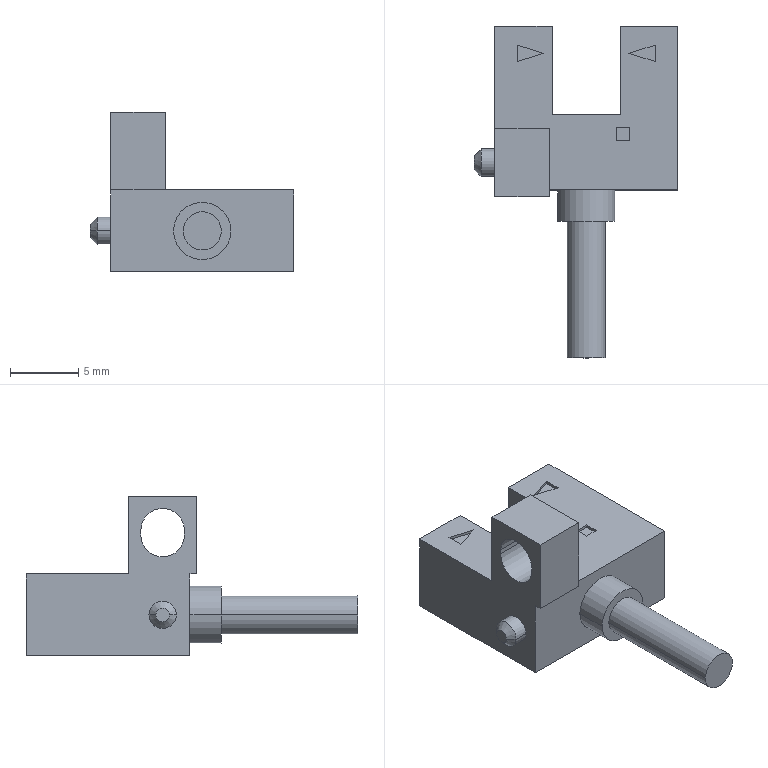Part | SolidWorks | features BaseBody 1 | 1 solid | 81 faces | box 14.9 x 24.3 x 11.7 mm | volume 940.552 mm3 | plane 71 | cylinder 8 | cone 2 | commonest cylinder face diameters 2 x2 2.8 x2 3.2 x2 4.2 x2